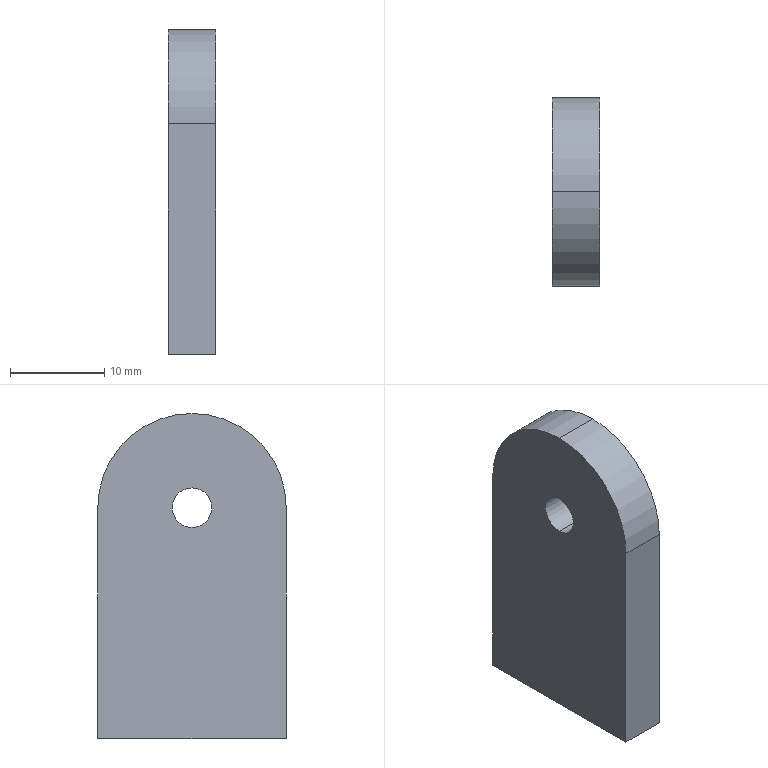Part | SolidWorks | features 3DProfileFeature 1, Extrusion 1, HoleWzd 1 | 1 solid | 9 faces | box 5 x 20 x 34.5 mm | volume 3166 mm3 | plane 5 | cylinder 4 | commonest cylinder face diameters 4.2 x2 20 x2
STEP:
#1=CARTESIAN_POINT('',(2.5,200.,37.4));
#2=VERTEX_POINT('',#1);
#3=CARTESIAN_POINT('',(2.5,200.,41.6));
#4=VERTEX_POINT('',#3);
#5=CARTESIAN_POINT('',(2.5,200.,39.5));
#6=DIRECTION('',(-1.,0.,0.));
#7=DIRECTION('',(0.,0.,1.));
#8=AXIS2_PLACEMENT_3D('',#5,#6,#7);
#9=CIRCLE('',#8,2.1);
#10=EDGE_CURVE('',#2,#4,#9,.T.);
#11=ORIENTED_EDGE('',*,*,#10,.F.);
#12=CARTESIAN_POINT('',(-2.5,200.,37.4));
#13=VERTEX_POINT('',#12);
#14=CARTESIAN_POINT('',(-2.5,200.,37.4));
#15=DIRECTION('',(-1.,0.,0.));
#16=VECTOR('',#15,1000.);
#17=LINE('',#14,#16);
#18=EDGE_CURVE('',#2,#13,#17,.T.);
#19=ORIENTED_EDGE('',*,*,#18,.T.);
#20=CARTESIAN_POINT('',(-2.5,200.,41.6));
#21=VERTEX_POINT('',#20);
#22=CARTESIAN_POINT('',(-2.5,200.,39.5));
#23=DIRECTION('',(-1.,0.,0.));
#24=DIRECTION('',(0.,0.,1.));
#25=AXIS2_PLACEMENT_3D('',#22,#23,#24);
#26=CIRCLE('',#25,2.1);
#27=EDGE_CURVE('',#13,#21,#26,.T.);
#28=ORIENTED_EDGE('',*,*,#27,.T.);
#29=CARTESIAN_POINT('',(-2.5,200.,41.6));
#30=DIRECTION('',(-1.,0.,0.));
#31=VECTOR('',#30,1000.);
#32=LINE('',#29,#31);
#33=EDGE_CURVE('',#4,#21,#32,.T.);
#34=ORIENTED_EDGE('',*,*,#33,.F.);
#35=EDGE_LOOP('',(#11,#19,#28,#34));
#36=FACE_OUTER_BOUND('',#35,.T.);
#37=CARTESIAN_POINT('',(-2.5,200.,39.5));
#38=DIRECTION('',(-1.,0.,0.));
#39=DIRECTION('',(0.,0.,1.));
#40=AXIS2_PLACEMENT_3D('',#37,#38,#39);
#41=CYLINDRICAL_SURFACE('',#40,2.1);
#42=ADVANCED_FACE('',(#36),#41,.F.);
#43=CARTESIAN_POINT('',(2.5,200.,49.5));
#44=VERTEX_POINT('',#43);
#45=CARTESIAN_POINT('',(2.5,190.,39.5));
#46=VERTEX_POINT('',#45);
#47=CARTESIAN_POINT('',(2.5,200.,39.5));
#48=DIRECTION('',(1.,0.,0.));
#49=DIRECTION('',(0.,0.,-1.));
#50=AXIS2_PLACEMENT_3D('',#47,#48,#49);
#51=CIRCLE('',#50,10.);
#52=EDGE_CURVE('',#44,#46,#51,.T.);
#53=ORIENTED_EDGE('',*,*,#52,.F.);
#54=CARTESIAN_POINT('',(-2.5,200.,49.5));
#55=VERTEX_POINT('',#54);
#56=CARTESIAN_POINT('',(2.5,200.,49.5));
#57=DIRECTION('',(-1.,0.,0.));
#58=VECTOR('',#57,1000.);
#59=LINE('',#56,#58);
#60=EDGE_CURVE('',#44,#55,#59,.T.);
#61=ORIENTED_EDGE('',*,*,#60,.T.);
#62=CARTESIAN_POINT('',(-2.5,190.,39.5));
#63=VERTEX_POINT('',#62);
#64=CARTESIAN_POINT('',(-2.5,200.,39.5));
#65=DIRECTION('',(1.,0.,0.));
#66=DIRECTION('',(0.,0.,-1.));
#67=AXIS2_PLACEMENT_3D('',#64,#65,#66);
#68=CIRCLE('',#67,10.);
#69=EDGE_CURVE('',#55,#63,#68,.T.);
#70=ORIENTED_EDGE('',*,*,#69,.T.);
#71=CARTESIAN_POINT('',(2.5,190.,39.5));
#72=DIRECTION('',(-1.,0.,0.));
#73=VECTOR('',#72,1000.);
#74=LINE('',#71,#73);
#75=EDGE_CURVE('',#46,#63,#74,.T.);
#76=ORIENTED_EDGE('',*,*,#75,.F.);
#77=EDGE_LOOP('',(#53,#61,#70,#76));
#78=FACE_OUTER_BOUND('',#77,.T.);
#79=CARTESIAN_POINT('',(2.5,200.,39.5));
#80=DIRECTION('',(-1.,0.,0.));
#81=DIRECTION('',(0.,0.,1.));
#82=AXIS2_PLACEMENT_3D('',#79,#80,#81);
#83=CYLINDRICAL_SURFACE('',#82,10.);
#84=ADVANCED_FACE('',(#78),#83,.T.);
#85=CARTESIAN_POINT('',(-2.5,190.,15.));
#86=VERTEX_POINT('',#85);
#87=CARTESIAN_POINT('',(-2.5,210.,15.));
#88=VERTEX_POINT('',#87);
#89=CARTESIAN_POINT('',(-2.5,210.,15.));
#90=DIRECTION('',(0.,1.,0.));
#91=VECTOR('',#90,1000.);
#92=LINE('',#89,#91);
#93=EDGE_CURVE('',#86,#88,#92,.T.);
#94=ORIENTED_EDGE('',*,*,#93,.F.);
#95=CARTESIAN_POINT('',(-2.5,190.,15.));
#96=DIRECTION('',(0.,0.,-1.));
#97=VECTOR('',#96,1000.);
#98=LINE('',#95,#97);
#99=EDGE_CURVE('',#63,#86,#98,.T.);
#100=ORIENTED_EDGE('',*,*,#99,.F.);
#101=ORIENTED_EDGE('',*,*,#69,.F.);
#102=CARTESIAN_POINT('',(-2.5,210.,39.5));
#103=VERTEX_POINT('',#102);
#104=CARTESIAN_POINT('',(-2.5,200.,39.5));
#105=DIRECTION('',(1.,0.,0.));
#106=DIRECTION('',(0.,0.,-1.));
#107=AXIS2_PLACEMENT_3D('',#104,#105,#106);
#108=CIRCLE('',#107,10.);
#109=EDGE_CURVE('',#103,#55,#108,.T.);
#110=ORIENTED_EDGE('',*,*,#109,.F.);
#111=CARTESIAN_POINT('',(-2.5,210.,15.));
#112=DIRECTION('',(0.,0.,1.));
#113=VECTOR('',#112,1000.);
#114=LINE('',#111,#113);
#115=EDGE_CURVE('',#88,#103,#114,.T.);
#116=ORIENTED_EDGE('',*,*,#115,.F.);
#117=EDGE_LOOP('',(#94,#100,#101,#110,#116));
#118=FACE_OUTER_BOUND('',#117,.T.);
#119=CARTESIAN_POINT('',(-2.5,200.,39.5));
#120=DIRECTION('',(-1.,0.,0.));
#121=DIRECTION('',(0.,0.,1.));
#122=AXIS2_PLACEMENT_3D('',#119,#120,#121);
#123=CIRCLE('',#122,2.1);
#124=EDGE_CURVE('',#21,#13,#123,.T.);
#125=ORIENTED_EDGE('',*,*,#124,.F.);
#126=ORIENTED_EDGE('',*,*,#27,.F.);
#127=EDGE_LOOP('',(#125,#126));
#128=FACE_BOUND('',#127,.T.);
#129=CARTESIAN_POINT('',(-2.5,200.,39.5));
#130=DIRECTION('',(1.,0.,0.));
#131=DIRECTION('',(0.,0.,-1.));
#132=AXIS2_PLACEMENT_3D('',#129,#130,#131);
#133=PLANE('',#132);
#134=ADVANCED_FACE('',(#118,#128),#133,.F.);
#135=ORIENTED_EDGE('',*,*,#93,.T.);
#136=CARTESIAN_POINT('',(2.5,210.,15.));
#137=VERTEX_POINT('',#136);
#138=CARTESIAN_POINT('',(2.5,210.,15.));
#139=DIRECTION('',(-1.,0.,0.));
#140=VECTOR('',#139,1000.);
#141=LINE('',#138,#140);
#142=EDGE_CURVE('',#137,#88,#141,.T.);
#143=ORIENTED_EDGE('',*,*,#142,.F.);
#144=CARTESIAN_POINT('',(2.5,190.,15.));
#145=VERTEX_POINT('',#144);
#146=CARTESIAN_POINT('',(2.5,210.,15.));
#147=DIRECTION('',(0.,1.,0.));
#148=VECTOR('',#147,1000.);
#149=LINE('',#146,#148);
#150=EDGE_CURVE('',#145,#137,#149,.T.);
#151=ORIENTED_EDGE('',*,*,#150,.F.);
#152=CARTESIAN_POINT('',(2.5,190.,15.));
#153=DIRECTION('',(-1.,0.,0.));
#154=VECTOR('',#153,1000.);
#155=LINE('',#152,#154);
#156=EDGE_CURVE('',#145,#86,#155,.T.);
#157=ORIENTED_EDGE('',*,*,#156,.T.);
#158=EDGE_LOOP('',(#135,#143,#151,#157));
#159=FACE_OUTER_BOUND('',#158,.T.);
#160=CARTESIAN_POINT('',(2.5,210.,15.));
#161=DIRECTION('',(0.,0.,1.));
#162=DIRECTION('',(1.,0.,0.));
#163=AXIS2_PLACEMENT_3D('',#160,#161,#162);
#164=PLANE('',#163);
#165=ADVANCED_FACE('',(#159),#164,.F.);
#166=ORIENTED_EDGE('',*,*,#115,.T.);
#167=CARTESIAN_POINT('',(2.5,210.,39.5));
#168=VERTEX_POINT('',#167);
#169=CARTESIAN_POINT('',(2.5,210.,39.5));
#170=DIRECTION('',(-1.,0.,0.));
#171=VECTOR('',#170,1000.);
#172=LINE('',#169,#171);
#173=EDGE_CURVE('',#168,#103,#172,.T.);
#174=ORIENTED_EDGE('',*,*,#173,.F.);
#175=CARTESIAN_POINT('',(2.5,210.,15.));
#176=DIRECTION('',(0.,0.,1.));
#177=VECTOR('',#176,1000.);
#178=LINE('',#175,#177);
#179=EDGE_CURVE('',#137,#168,#178,.T.);
#180=ORIENTED_EDGE('',*,*,#179,.F.);
#181=ORIENTED_EDGE('',*,*,#142,.T.);
#182=EDGE_LOOP('',(#166,#174,#180,#181));
#183=FACE_OUTER_BOUND('',#182,.T.);
#184=CARTESIAN_POINT('',(2.5,210.,15.));
#185=DIRECTION('',(0.,-1.,0.));
#186=DIRECTION('',(0.,0.,-1.));
#187=AXIS2_PLACEMENT_3D('',#184,#185,#186);
#188=PLANE('',#187);
#189=ADVANCED_FACE('',(#183),#188,.F.);
#190=ORIENTED_EDGE('',*,*,#60,.F.);
#191=CARTESIAN_POINT('',(2.5,200.,39.5));
#192=DIRECTION('',(1.,0.,0.));
#193=DIRECTION('',(0.,0.,-1.));
#194=AXIS2_PLACEMENT_3D('',#191,#192,#193);
#195=CIRCLE('',#194,10.);
#196=EDGE_CURVE('',#168,#44,#195,.T.);
#197=ORIENTED_EDGE('',*,*,#196,.F.);
#198=ORIENTED_EDGE('',*,*,#173,.T.);
#199=ORIENTED_EDGE('',*,*,#109,.T.);
#200=EDGE_LOOP('',(#190,#197,#198,#199));
#201=FACE_OUTER_BOUND('',#200,.T.);
#202=CARTESIAN_POINT('',(2.5,200.,39.5));
#203=DIRECTION('',(-1.,0.,0.));
#204=DIRECTION('',(0.,0.,1.));
#205=AXIS2_PLACEMENT_3D('',#202,#203,#204);
#206=CYLINDRICAL_SURFACE('',#205,10.);
#207=ADVANCED_FACE('',(#201),#206,.T.);
#208=ORIENTED_EDGE('',*,*,#99,.T.);
#209=ORIENTED_EDGE('',*,*,#156,.F.);
#210=CARTESIAN_POINT('',(2.5,190.,15.));
#211=DIRECTION('',(0.,0.,-1.));
#212=VECTOR('',#211,1000.);
#213=LINE('',#210,#212);
#214=EDGE_CURVE('',#46,#145,#213,.T.);
#215=ORIENTED_EDGE('',*,*,#214,.F.);
#216=ORIENTED_EDGE('',*,*,#75,.T.);
#217=EDGE_LOOP('',(#208,#209,#215,#216));
#218=FACE_OUTER_BOUND('',#217,.T.);
#219=CARTESIAN_POINT('',(2.5,190.,15.));
#220=DIRECTION('',(0.,1.,0.));
#221=DIRECTION('',(0.,0.,1.));
#222=AXIS2_PLACEMENT_3D('',#219,#220,#221);
#223=PLANE('',#222);
#224=ADVANCED_FACE('',(#218),#223,.F.);
#225=CARTESIAN_POINT('',(2.5,200.,39.5));
#226=DIRECTION('',(-1.,0.,0.));
#227=DIRECTION('',(0.,0.,1.));
#228=AXIS2_PLACEMENT_3D('',#225,#226,#227);
#229=CIRCLE('',#228,2.1);
#230=EDGE_CURVE('',#4,#2,#229,.T.);
#231=ORIENTED_EDGE('',*,*,#230,.T.);
#232=ORIENTED_EDGE('',*,*,#10,.T.);
#233=EDGE_LOOP('',(#231,#232));
#234=FACE_BOUND('',#233,.T.);
#235=ORIENTED_EDGE('',*,*,#150,.T.);
#236=ORIENTED_EDGE('',*,*,#179,.T.);
#237=ORIENTED_EDGE('',*,*,#196,.T.);
#238=ORIENTED_EDGE('',*,*,#52,.T.);
#239=ORIENTED_EDGE('',*,*,#214,.T.);
#240=EDGE_LOOP('',(#235,#236,#237,#238,#239));
#241=FACE_OUTER_BOUND('',#240,.T.);
#242=CARTESIAN_POINT('',(2.5,200.,39.5));
#243=DIRECTION('',(1.,0.,0.));
#244=DIRECTION('',(0.,0.,-1.));
#245=AXIS2_PLACEMENT_3D('',#242,#243,#244);
#246=PLANE('',#245);
#247=ADVANCED_FACE('',(#234,#241),#246,.T.);
#248=ORIENTED_EDGE('',*,*,#18,.F.);
#249=ORIENTED_EDGE('',*,*,#230,.F.);
#250=ORIENTED_EDGE('',*,*,#33,.T.);
#251=ORIENTED_EDGE('',*,*,#124,.T.);
#252=EDGE_LOOP('',(#248,#249,#250,#251));
#253=FACE_OUTER_BOUND('',#252,.T.);
#254=CARTESIAN_POINT('',(-2.5,200.,39.5));
#255=DIRECTION('',(-1.,0.,0.));
#256=DIRECTION('',(0.,0.,1.));
#257=AXIS2_PLACEMENT_3D('',#254,#255,#256);
#258=CYLINDRICAL_SURFACE('',#257,2.1);
#259=ADVANCED_FACE('',(#253),#258,.F.);
#260=CLOSED_SHELL('',(#42,#84,#134,#165,#189,#207,#224,#247,#259));
#261=MANIFOLD_SOLID_BREP('',#260);
#262=CARTESIAN_POINT('',(0.,0.,0.));
#263=DIRECTION('',(0.,0.,1.));
#264=DIRECTION('',(1.,0.,0.));
#265=AXIS2_PLACEMENT_3D('',#262,#263,#264);
#266=(LENGTH_UNIT()NAMED_UNIT(*)SI_UNIT(.MILLI.,.METRE.));
#267=UNCERTAINTY_MEASURE_WITH_UNIT(LENGTH_MEASURE(0.00001),#266,'','');
#268=(NAMED_UNIT(*)PLANE_ANGLE_UNIT()SI_UNIT($,.RADIAN.));
#269=(NAMED_UNIT(*)SI_UNIT($,.STERADIAN.)SOLID_ANGLE_UNIT());
#270=(GEOMETRIC_REPRESENTATION_CONTEXT(3)GLOBAL_UNCERTAINTY_ASSIGNED_CONTEXT((#267))GLOBAL_UNIT_ASSIGNED_CONTEXT((#266,#268,#269))REPRESENTATION_CONTEXT('',''));
#271=ADVANCED_BREP_SHAPE_REPRESENTATION('',(#261,#265),#270);